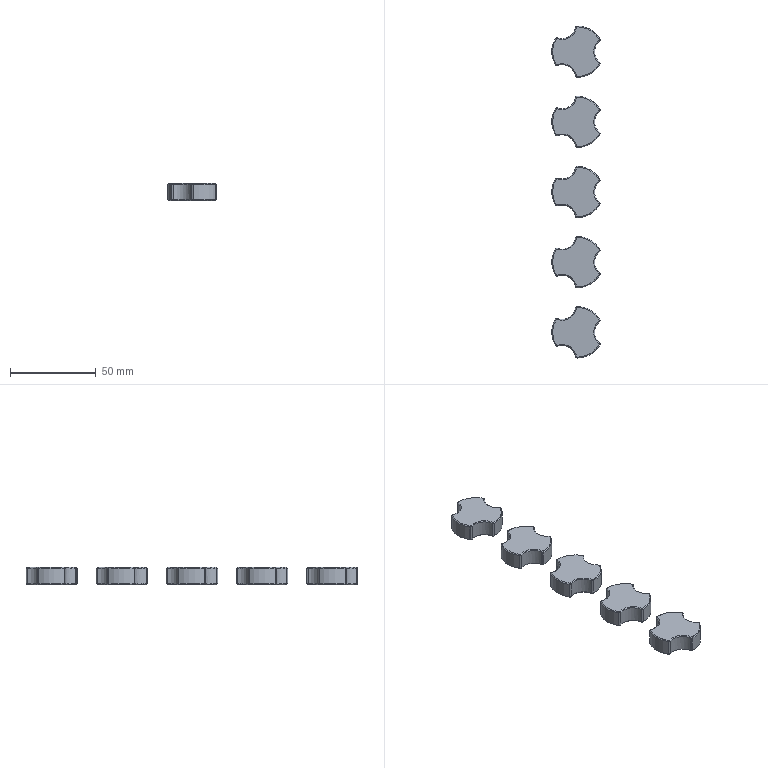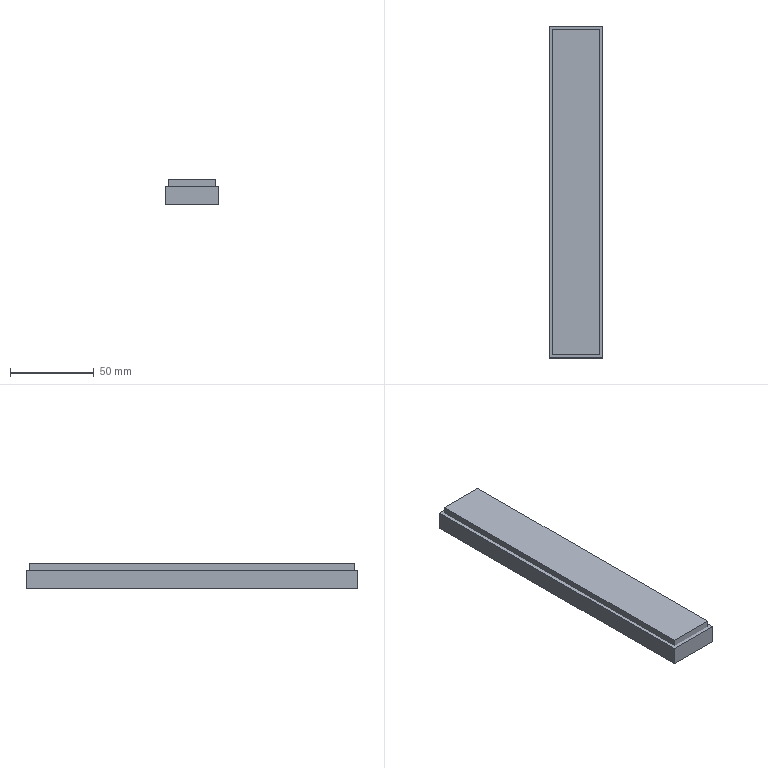CAM job | NX | 3-axis milling | part box 28.194 x 194 x 10 mm | stock box 32.194 x 198 x 15 mm
Tools:
number,name,description,diameter,corner_radius,flute_length,length,flutes
19,D80,Milling Tool-5 Parameters,80.0,0.0,50.0,75.0,2
15,D10,Milling Tool-5 Parameters,10.0,0.0,50.0,75.0,2
14,D10JING,Milling Tool-5 Parameters,10.0,0.0,50.0,75.0,2
16,D2,Milling Tool-5 Parameters,2.0,0.0,50.0,75.0,2
1,D6A45,Milling Tool-5 Parameters,6.0,0.0,50.0,75.0,2
Operations:
program,operation,operation_type,tool,method,geometry_group,spindle_rpm,surface_speed,feed_per_tooth,feed_cut,feed_plunge,cut_length_mm,path_length_mm,cut_time_min,machine_time_min
1,FLOOR_WALL,VolumeBased25DMillingOperation,D80,METHOD,A,6500.0,1633.0,0.1154,1500.0,100.0,294.0,348.0,0.196,0.2014
1,ZLEVEL_PROFILE_COPY_1,ZLevelMilling,D10,METHOD,A,9500.0,298.0,0.1842,3500.0,1000.0,7401.468,8180.281,2.285,2.363
1,ZLEVEL_PROFILE_COPY_1_COPY,ZLevelMilling,D10JING,METHOD,A,9500.0,298.0,0.0632,1200.0,1000.0,673.136,1657.12,0.5631,0.6615
1,HOLE_MILLING,CylinderMilling,D2,METHOD,A,9500.0,89.0,0.0605,1150.0,100.0,648.286,1144.786,0.5637,0.6134
1,PLANAR_MILL_COPY_COPY_COPY_COPY,PlanarMilling,D6A45,METHOD,A,9500.0,179.0,0.0658,1250.0,100.0,583.222,1471.11,0.4666,0.5554
1,刀补17,CylinderMilling,D2,METHOD,A,9500.0,89.0,0.0605,1150.0,100.0,86.067,582.567,0.0748,0.1245
2,FLOOR_WALL_COPY,VolumeBased25DMillingOperation,D80,METHOD,B,6500.0,1633.0,0.1154,1500.0,100.0,2900,5951.002,1.933,2.238
2,PLANAR_MILL_COPY_COPY_COPY_COPY_COPY,PlanarMilling,D6A45,METHOD,B,9500.0,179.0,0.0658,1250.0,100.0,547.279,1017.297,0.4378,0.4848